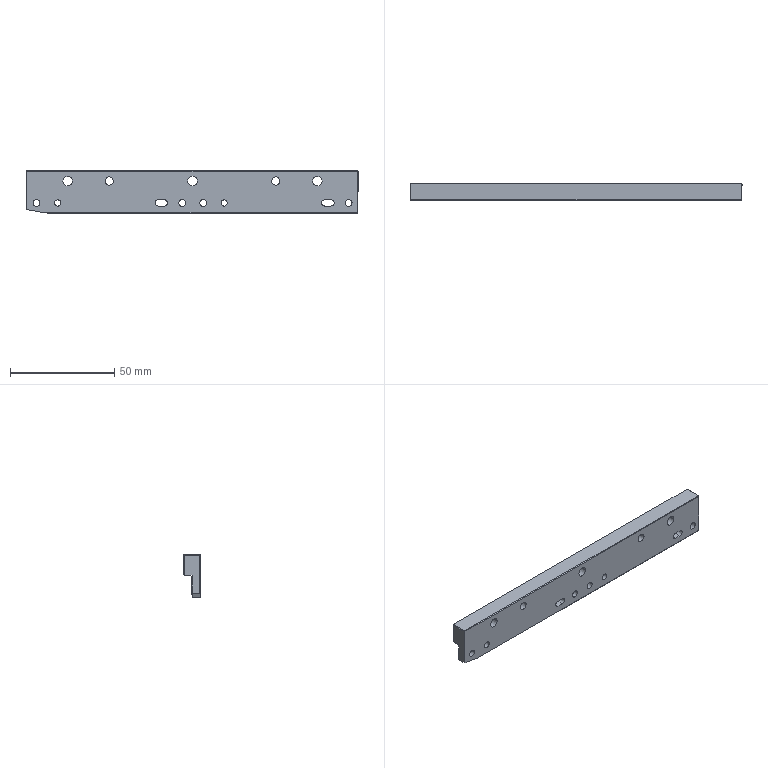Part | NX | 1 solid | 70 faces | box 159.5 x 8 x 20.5 mm | volume 18475 mm3 | cylinder 28 | plane 24 | cone 18 | commonest cylinder face diameters 3 x10 3.3 x8 4.5 x6 4 x4